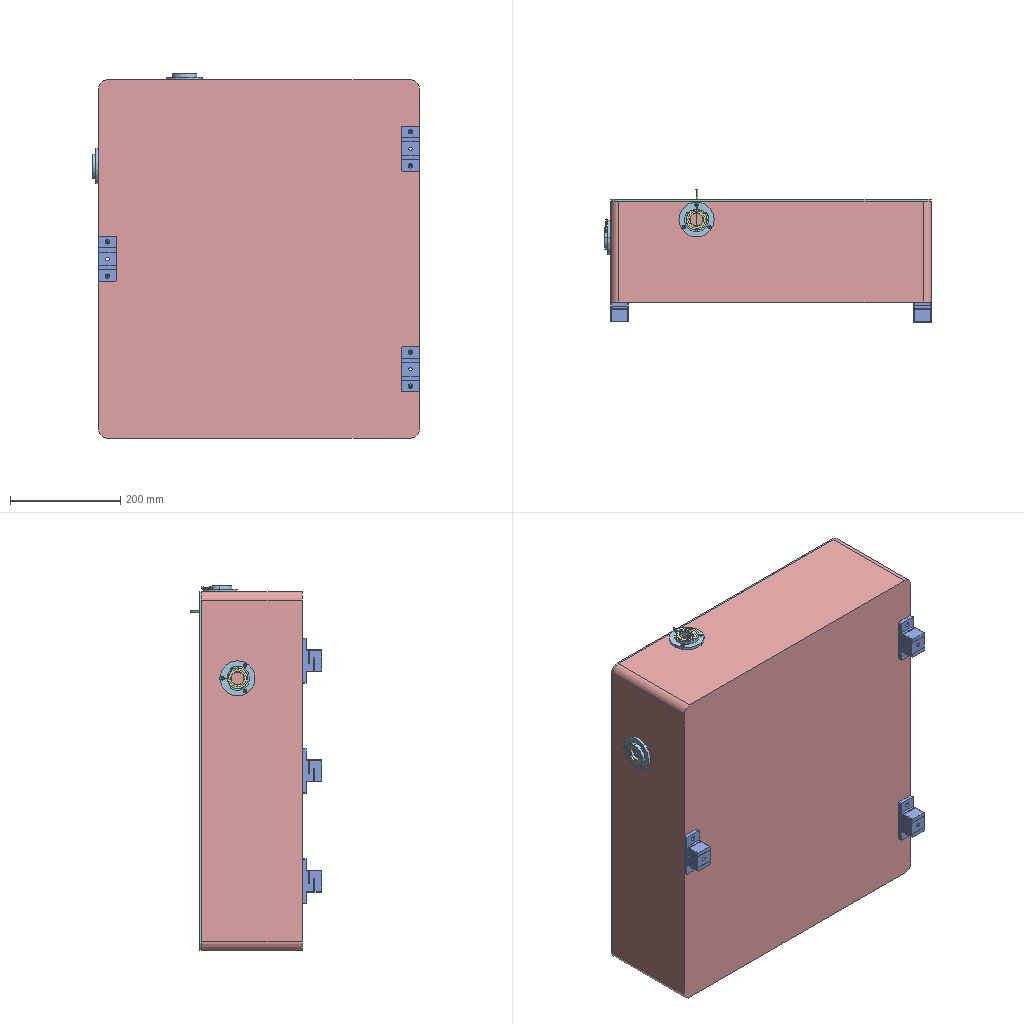Assembly | SolidWorks | 11 different items | 16 placed | box 593 x 239 x 661 mm
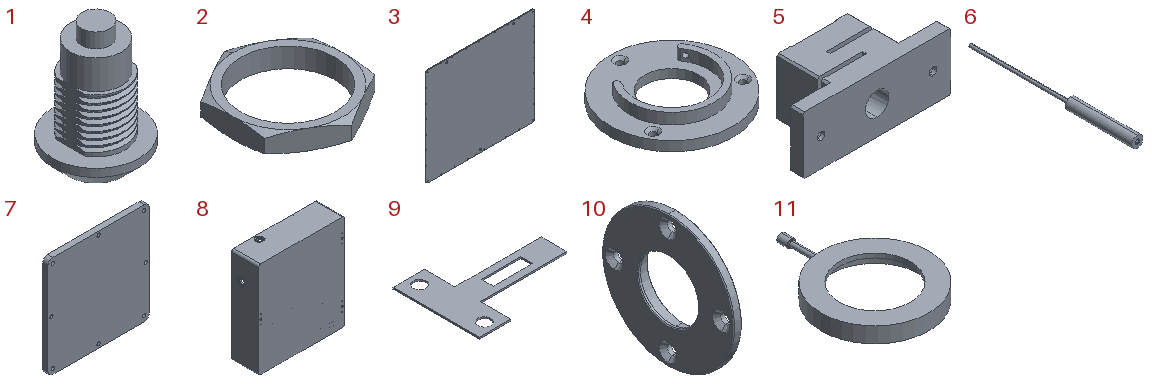Parts list (item | quantity | size | volume | features):
1 | x1 | 17.8 x 17.8 x 25 mm | 2223 mm3 | features ICE 7, Chamfer 1, Extrusion 1, Fillet 1, SweepThread 1
2 | x1 | 14 x 16.166 x 2.5 mm | 137.79 mm3 | features Extrusion 1, RevCut 1
3 | x1 | 650 x 3.5 x 582 mm | 1318505 mm3 | features Extrusion 1, HoleWzd 1, ICE 1
4 | x2 | 64 x 64 x 10.7 mm | 13896 mm3 | features Fillet 3, ICE 3, HoleWzd 2, Extrusion 1
5 | x3 | 82 x 35.5 x 32 mm | 46922 mm3 | features ICE 6, Chamfer 1, Extrusion 1
6 | x1 | 10 x 150 x 10 mm | 5247 mm3 | features Extrusion 1, HoleWzd 1, ICE 1
7 | x1 | 99 x 5 x 99 mm | 48448 mm3 | features Extrusion 1, Fillet 1, HoleWzd 1
8 | x1 | 582 x 183 x 650 mm | 11923446 mm3 | features ICE 20, HoleWzd 13, Fillet 6, Chamfer 1, Extrusion 1, Shell 1
9 | x1 | 30 x 22 x 0.4115 mm | 112.299 mm3 | features BaseBody 1
10 | x2 | 5.5 x 48 x 48 mm | 4296 mm3 | features Chamfer 2, ICE 1, Revolution 1
11 | x2 | 38 x 52.6 x 5.5 mm | 2350 mm3 | features BaseBody 2
Mates (type | each side: item.copy, entity, surface, feature):
Coincident | 8.1 face plane Boss-Extrude1 | 5.1 face plane Boss-Extrude1
Concentric | 8.1 face cylinder M4 Tapped Hole1 | 5.1 face cylinder Cut-Extrude2 | 2 times
Coincident | 8.1 face plane Boss-Extrude1 | 5.2 face plane Boss-Extrude1
Coincident | 8.1 face plane Boss-Extrude1 | 5.3 face plane Boss-Extrude1
Concentric | 8.1 face cylinder M4 Tapped Hole1 | 5.3 face cylinder Cut-Extrude2 | 2 times
Concentric | 8.1 edge | 5.2 face cylinder Cut-Extrude2 | 2 times
Coincident | 8.1 face plane Boss-Extrude2 | 6.1 face plane Boss-Extrude1
Coincident | 8.1 face plane Shell1 | 9.1 face plane Input1
Parallel | 8.1 face plane Shell1 | 9.1 edge
Coincident | 8.1 face plane Boss-Extrude1 | 3.1 face plane Boss-Extrude1
Concentric | 8.1 face cylinder Cut-Extrude1 | 3.1 face cylinder Cut-Extrude1 | 2 times
Coincident | 8.1 face plane Cut-Extrude11 | 7.1 face plane Boss-Extrude1
DistanceDim | 8.1 face plane Cut-Extrude11 | 7.1 face plane Boss-Extrude1
DistanceDim | 7.1 face plane Boss-Extrude1 | 8.1 face plane Cut-Extrude11
Concentric | 8.1 face cylinder Cut-Extrude5 | 10.1 face cylinder Revolve1
Coincident | 8.1 face plane Cut-Extrude6 | 10.1 face plane Revolve1
Concentric | 8.1 face cylinder M3 Tapped Hole3 | 10.1 face cone Chamfer1
Concentric | 8.1 face cylinder Cut-Extrude8 | 10.2 face cylinder Revolve1
Coincident | 8.1 face plane Cut-Extrude9 | 10.2 face plane Revolve1
Concentric | 8.1 face cylinder M3 Tapped Hole5 | 10.2 face cone Chamfer1
Concentric | 8.1 face cylinder Cut-Extrude3 | 1.1 face cylinder Boss-Extrude3
Coincident | 8.1 face plane Cut-Extrude4 | 1.1 face plane Boss-Extrude1
Concentric | 1.1 face cylinder Boss-Extrude3 | 2.1 face cylinder Boss-Extrude1
Coincident | 8.1 face plane Shell1 | 2.1 face plane Boss-Extrude1
Coincident | 8.1 face plane Boss-Extrude1 | 4.1 face plane Boss-Extrude1
Concentric | 8.1 face cylinder Cut-Extrude8 | 4.1 face cylinder Boss-Extrude1
Concentric | 8.1 face cylinder M3 Tapped Hole4 | 4.1 face cone CSK for M3 Flat Head Machine Screw1
Concentric | 8.1 face cylinder Cut-Extrude5 | 4.2 face cylinder Boss-Extrude1
Coincident | 8.1 face plane Boss-Extrude1 | 4.2 face plane Boss-Extrude1
Concentric | 8.1 face cylinder M3 Tapped Hole2 | 4.2 face cone CSK for M3 Flat Head Machine Screw1
Concentric | 4.1 face cylinder Boss-Extrude2 | 11.1 face cylinder Input2
Coincident | 4.1 face plane Boss-Extrude1 | 11.1 face plane Input2
Concentric | 4.2 face cylinder Boss-Extrude2 | 11.2 face cylinder Input2
Coincident | 4.2 face plane Boss-Extrude1 | 11.2 face plane Input2